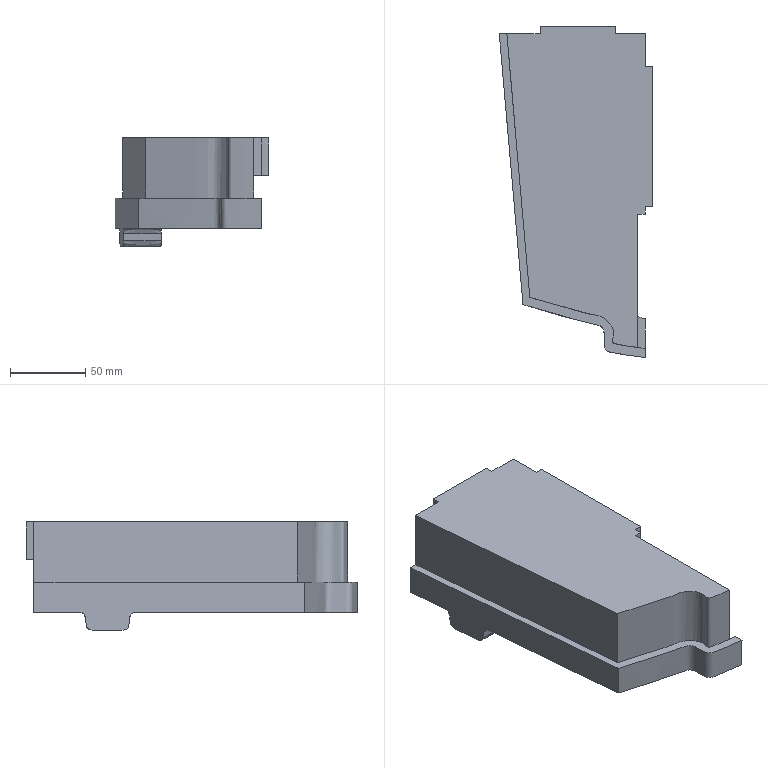Part | NX | features solid 2 | 1 solid | 41 faces | box 102.12 x 220.41 x 72 mm | volume 614371 mm3 | plane 23 | spline 14 | cylinder 4 | commonest cylinder face diameters 25 x2 30 x2